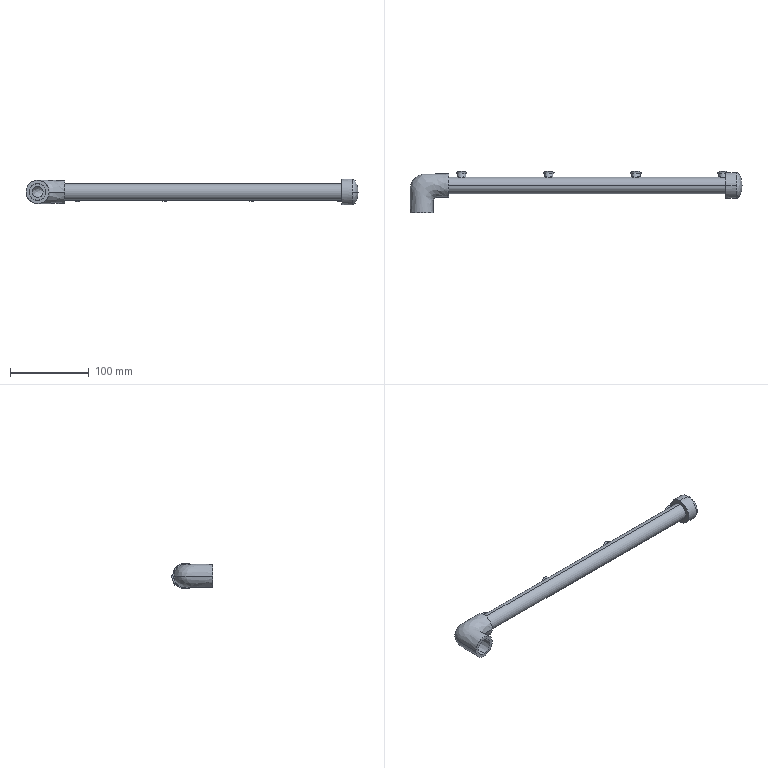Part | SolidWorks | 7 solids | 155 faces | box 422.844 x 53.25 x 32.766 mm | volume 119416 mm3 | cylinder 70 | plane 39 | cone 30 | torus 8 | spline 8 | commonest cylinder face diameters 8 x16 6.476 x8 10 x8 10.8 x8 10.935 x8 12.15 x8